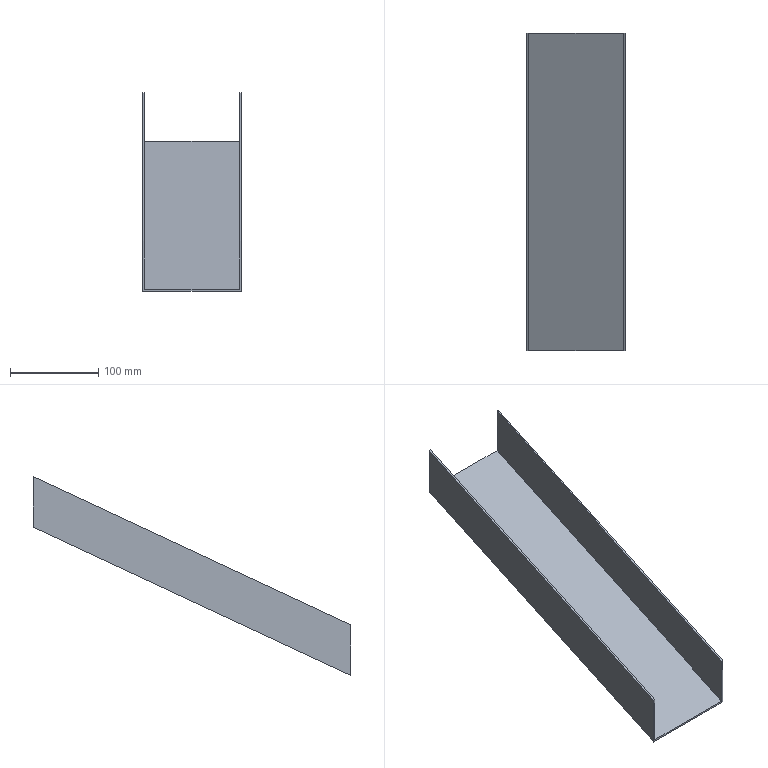Part | NX | features solid 2 | 1 solid | 10 faces | box 111.182 x 360 x 225.246 mm | volume 167770 mm3 | plane 10
STEP:
#1=CARTESIAN_POINT('',(100.,-105.,-113.856));
#2=VERTEX_POINT('',#1);
#3=CARTESIAN_POINT('',(102.,-105.,-113.856));
#4=VERTEX_POINT('',#3);
#5=CARTESIAN_POINT('',(121.182,-105.,-113.856));
#6=DIRECTION('',(-1.,0.,0.));
#7=VECTOR('',#6,1000.);
#8=LINE('',#5,#7);
#9=EDGE_CURVE('',#2,#4,#8,.F.);
#10=ORIENTED_EDGE('',*,*,#9,.F.);
#11=CARTESIAN_POINT('',(100.,-465.,-281.727));
#12=VERTEX_POINT('',#11);
#13=CARTESIAN_POINT('',(100.,-232.92,-173.506));
#14=DIRECTION('',(0.,-0.9063,-0.4226));
#15=VECTOR('',#14,1000.);
#16=LINE('',#13,#15);
#17=EDGE_CURVE('',#2,#12,#16,.T.);
#18=ORIENTED_EDGE('',*,*,#17,.T.);
#19=CARTESIAN_POINT('',(102.,-465.,-281.727));
#20=VERTEX_POINT('',#19);
#21=CARTESIAN_POINT('',(110.,-465.,-281.727));
#22=DIRECTION('',(-1.,0.,0.));
#23=VECTOR('',#22,1000.);
#24=LINE('',#21,#23);
#25=EDGE_CURVE('',#12,#20,#24,.F.);
#26=ORIENTED_EDGE('',*,*,#25,.T.);
#27=CARTESIAN_POINT('',(102.,-283.317,-197.007));
#28=DIRECTION('',(0.,-0.9063,-0.4226));
#29=VECTOR('',#28,1000.);
#30=LINE('',#27,#29);
#31=EDGE_CURVE('',#4,#20,#30,.T.);
#32=ORIENTED_EDGE('',*,*,#31,.F.);
#33=EDGE_LOOP('',(#10,#18,#26,#32));
#34=FACE_BOUND('',#33,.T.);
#35=CARTESIAN_POINT('',(110.,-161.131,-140.03));
#36=DIRECTION('',(0.,0.4226,-0.9063));
#37=DIRECTION('',(0.,-0.9063,-0.4226));
#38=AXIS2_PLACEMENT_3D('',#35,#36,#37);
#39=PLANE('',#38);
#40=ADVANCED_FACE('',(#34),#39,.F.);
#41=CARTESIAN_POINT('',(102.,-105.,-169.025));
#42=VERTEX_POINT('',#41);
#43=CARTESIAN_POINT('',(102.,-465.,-336.896));
#44=VERTEX_POINT('',#43);
#45=CARTESIAN_POINT('',(102.,-7.673,-123.64));
#46=DIRECTION('',(0.,-0.9063,-0.4226));
#47=VECTOR('',#46,1000.);
#48=LINE('',#45,#47);
#49=EDGE_CURVE('',#42,#44,#48,.T.);
#50=ORIENTED_EDGE('',*,*,#49,.F.);
#51=CARTESIAN_POINT('',(102.,-105.,0.000000171));
#52=DIRECTION('',(0.,0.,1.));
#53=VECTOR('',#52,1000.);
#54=LINE('',#51,#53);
#55=EDGE_CURVE('',#42,#4,#54,.T.);
#56=ORIENTED_EDGE('',*,*,#55,.T.);
#57=ORIENTED_EDGE('',*,*,#31,.T.);
#58=CARTESIAN_POINT('',(102.,-465.,-242.322));
#59=DIRECTION('',(0.,0.,1.));
#60=VECTOR('',#59,1000.);
#61=LINE('',#58,#60);
#62=EDGE_CURVE('',#44,#20,#61,.T.);
#63=ORIENTED_EDGE('',*,*,#62,.F.);
#64=EDGE_LOOP('',(#50,#56,#57,#63));
#65=FACE_BOUND('',#64,.T.);
#66=CARTESIAN_POINT('',(102.,-262.186,-242.322));
#67=DIRECTION('',(-1.,0.,0.));
#68=DIRECTION('',(0.,0.,1.));
#69=AXIS2_PLACEMENT_3D('',#66,#67,#68);
#70=PLANE('',#69);
#71=ADVANCED_FACE('',(#65),#70,.F.);
#72=ORIENTED_EDGE('',*,*,#55,.F.);
#73=CARTESIAN_POINT('',(209.182,-105.,-169.025));
#74=VERTEX_POINT('',#73);
#75=CARTESIAN_POINT('',(121.182,-105.,-169.025));
#76=DIRECTION('',(1.,0.,0.));
#77=VECTOR('',#76,1000.);
#78=LINE('',#75,#77);
#79=EDGE_CURVE('',#42,#74,#78,.T.);
#80=ORIENTED_EDGE('',*,*,#79,.T.);
#81=CARTESIAN_POINT('',(209.182,-105.,-113.856));
#82=VERTEX_POINT('',#81);
#83=CARTESIAN_POINT('',(209.182,-105.,0.000000171));
#84=DIRECTION('',(0.,0.,1.));
#85=VECTOR('',#84,1000.);
#86=LINE('',#83,#85);
#87=EDGE_CURVE('',#74,#82,#86,.T.);
#88=ORIENTED_EDGE('',*,*,#87,.T.);
#89=CARTESIAN_POINT('',(211.182,-105.,-113.856));
#90=VERTEX_POINT('',#89);
#91=CARTESIAN_POINT('',(211.182,-105.,-113.856));
#92=DIRECTION('',(1.,0.,0.));
#93=VECTOR('',#92,1000.);
#94=LINE('',#91,#93);
#95=EDGE_CURVE('',#82,#90,#94,.T.);
#96=ORIENTED_EDGE('',*,*,#95,.T.);
#97=CARTESIAN_POINT('',(211.182,-105.,-171.232));
#98=VERTEX_POINT('',#97);
#99=CARTESIAN_POINT('',(211.182,-105.,0.000000171));
#100=DIRECTION('',(0.,0.,1.));
#101=VECTOR('',#100,1000.);
#102=LINE('',#99,#101);
#103=EDGE_CURVE('',#98,#90,#102,.T.);
#104=ORIENTED_EDGE('',*,*,#103,.F.);
#105=CARTESIAN_POINT('',(100.,-105.,-171.232));
#106=VERTEX_POINT('',#105);
#107=CARTESIAN_POINT('',(540.,-105.,-171.232));
#108=DIRECTION('',(1.,0.,0.));
#109=VECTOR('',#108,1000.);
#110=LINE('',#107,#109);
#111=EDGE_CURVE('',#106,#98,#110,.T.);
#112=ORIENTED_EDGE('',*,*,#111,.F.);
#113=CARTESIAN_POINT('',(100.,-105.,0.000000171));
#114=DIRECTION('',(0.,0.,1.));
#115=VECTOR('',#114,1000.);
#116=LINE('',#113,#115);
#117=EDGE_CURVE('',#106,#2,#116,.T.);
#118=ORIENTED_EDGE('',*,*,#117,.T.);
#119=ORIENTED_EDGE('',*,*,#9,.T.);
#120=EDGE_LOOP('',(#72,#80,#88,#96,#104,#112,#118,#119));
#121=FACE_BOUND('',#120,.T.);
#122=CARTESIAN_POINT('',(121.182,-105.,0.000000171));
#123=DIRECTION('',(0.,1.,0.));
#124=DIRECTION('',(0.,0.,1.));
#125=AXIS2_PLACEMENT_3D('',#122,#123,#124);
#126=PLANE('',#125);
#127=ADVANCED_FACE('',(#121),#126,.T.);
#128=ORIENTED_EDGE('',*,*,#17,.F.);
#129=ORIENTED_EDGE('',*,*,#117,.F.);
#130=CARTESIAN_POINT('',(100.,-465.,-339.102));
#131=VERTEX_POINT('',#130);
#132=CARTESIAN_POINT('',(100.,-6.828,-125.453));
#133=DIRECTION('',(0.,0.9063,0.4226));
#134=VECTOR('',#133,1000.);
#135=LINE('',#132,#134);
#136=EDGE_CURVE('',#131,#106,#135,.T.);
#137=ORIENTED_EDGE('',*,*,#136,.F.);
#138=CARTESIAN_POINT('',(100.,-465.,-85.));
#139=DIRECTION('',(0.,0.,-1.));
#140=VECTOR('',#139,1000.);
#141=LINE('',#138,#140);
#142=EDGE_CURVE('',#12,#131,#141,.T.);
#143=ORIENTED_EDGE('',*,*,#142,.F.);
#144=EDGE_LOOP('',(#128,#129,#137,#143));
#145=FACE_BOUND('',#144,.T.);
#146=CARTESIAN_POINT('',(100.,-90.,-480.));
#147=DIRECTION('',(-1.,0.,0.));
#148=DIRECTION('',(0.,0.,1.));
#149=AXIS2_PLACEMENT_3D('',#146,#147,#148);
#150=PLANE('',#149);
#151=ADVANCED_FACE('',(#145),#150,.T.);
#152=CARTESIAN_POINT('',(211.182,-465.,-339.102));
#153=VERTEX_POINT('',#152);
#154=CARTESIAN_POINT('',(-910.,-465.,-339.102));
#155=DIRECTION('',(1.,0.,0.));
#156=VECTOR('',#155,1000.);
#157=LINE('',#154,#156);
#158=EDGE_CURVE('',#131,#153,#157,.T.);
#159=ORIENTED_EDGE('',*,*,#158,.T.);
#160=CARTESIAN_POINT('',(211.182,-465.,-281.727));
#161=VERTEX_POINT('',#160);
#162=CARTESIAN_POINT('',(211.182,-465.,-85.));
#163=DIRECTION('',(0.,0.,-1.));
#164=VECTOR('',#163,1000.);
#165=LINE('',#162,#164);
#166=EDGE_CURVE('',#161,#153,#165,.T.);
#167=ORIENTED_EDGE('',*,*,#166,.F.);
#168=CARTESIAN_POINT('',(209.182,-465.,-281.727));
#169=VERTEX_POINT('',#168);
#170=CARTESIAN_POINT('',(211.182,-465.,-281.727));
#171=DIRECTION('',(-1.,0.,0.));
#172=VECTOR('',#171,1000.);
#173=LINE('',#170,#172);
#174=EDGE_CURVE('',#161,#169,#173,.T.);
#175=ORIENTED_EDGE('',*,*,#174,.T.);
#176=CARTESIAN_POINT('',(209.182,-465.,-336.896));
#177=VERTEX_POINT('',#176);
#178=CARTESIAN_POINT('',(209.182,-465.,-85.));
#179=DIRECTION('',(0.,0.,-1.));
#180=VECTOR('',#179,1000.);
#181=LINE('',#178,#180);
#182=EDGE_CURVE('',#169,#177,#181,.T.);
#183=ORIENTED_EDGE('',*,*,#182,.T.);
#184=CARTESIAN_POINT('',(140.,-465.,-336.896));
#185=DIRECTION('',(1.,0.,0.));
#186=VECTOR('',#185,1000.);
#187=LINE('',#184,#186);
#188=EDGE_CURVE('',#44,#177,#187,.T.);
#189=ORIENTED_EDGE('',*,*,#188,.F.);
#190=ORIENTED_EDGE('',*,*,#62,.T.);
#191=ORIENTED_EDGE('',*,*,#25,.F.);
#192=ORIENTED_EDGE('',*,*,#142,.T.);
#193=EDGE_LOOP('',(#159,#167,#175,#183,#189,#190,#191,#192));
#194=FACE_BOUND('',#193,.T.);
#195=CARTESIAN_POINT('',(-910.,-465.,-85.));
#196=DIRECTION('',(0.,-1.,0.));
#197=DIRECTION('',(0.,0.,-1.));
#198=AXIS2_PLACEMENT_3D('',#195,#196,#197);
#199=PLANE('',#198);
#200=ADVANCED_FACE('',(#194),#199,.T.);
#201=ORIENTED_EDGE('',*,*,#136,.T.);
#202=ORIENTED_EDGE('',*,*,#111,.T.);
#203=CARTESIAN_POINT('',(211.182,-6.828,-125.453));
#204=DIRECTION('',(0.,0.9063,0.4226));
#205=VECTOR('',#204,1000.);
#206=LINE('',#203,#205);
#207=EDGE_CURVE('',#153,#98,#206,.T.);
#208=ORIENTED_EDGE('',*,*,#207,.F.);
#209=ORIENTED_EDGE('',*,*,#158,.F.);
#210=EDGE_LOOP('',(#201,#202,#208,#209));
#211=FACE_BOUND('',#210,.T.);
#212=CARTESIAN_POINT('',(540.,-6.828,-125.453));
#213=DIRECTION('',(0.,0.4226,-0.9063));
#214=DIRECTION('',(0.,0.9063,0.4226));
#215=AXIS2_PLACEMENT_3D('',#212,#213,#214);
#216=PLANE('',#215);
#217=ADVANCED_FACE('',(#211),#216,.T.);
#218=ORIENTED_EDGE('',*,*,#188,.T.);
#219=CARTESIAN_POINT('',(209.182,-7.673,-123.64));
#220=DIRECTION('',(0.,-0.9063,-0.4226));
#221=VECTOR('',#220,1000.);
#222=LINE('',#219,#221);
#223=EDGE_CURVE('',#74,#177,#222,.T.);
#224=ORIENTED_EDGE('',*,*,#223,.F.);
#225=ORIENTED_EDGE('',*,*,#79,.F.);
#226=ORIENTED_EDGE('',*,*,#49,.T.);
#227=EDGE_LOOP('',(#218,#224,#225,#226));
#228=FACE_BOUND('',#227,.T.);
#229=CARTESIAN_POINT('',(140.,-7.673,-123.64));
#230=DIRECTION('',(0.,-0.4226,0.9063));
#231=DIRECTION('',(0.,-0.9063,-0.4226));
#232=AXIS2_PLACEMENT_3D('',#229,#230,#231);
#233=PLANE('',#232);
#234=ADVANCED_FACE('',(#228),#233,.T.);
#235=CARTESIAN_POINT('',(211.182,-57.284,-91.605));
#236=DIRECTION('',(0.,-0.9063,-0.4226));
#237=VECTOR('',#236,1000.);
#238=LINE('',#235,#237);
#239=EDGE_CURVE('',#90,#161,#238,.T.);
#240=ORIENTED_EDGE('',*,*,#239,.T.);
#241=ORIENTED_EDGE('',*,*,#166,.T.);
#242=ORIENTED_EDGE('',*,*,#207,.T.);
#243=ORIENTED_EDGE('',*,*,#103,.T.);
#244=EDGE_LOOP('',(#240,#241,#242,#243));
#245=FACE_BOUND('',#244,.T.);
#246=CARTESIAN_POINT('',(211.182,-100.,0.000000167));
#247=DIRECTION('',(-1.,0.,0.));
#248=DIRECTION('',(0.,-1.,0.));
#249=AXIS2_PLACEMENT_3D('',#246,#247,#248);
#250=PLANE('',#249);
#251=ADVANCED_FACE('',(#245),#250,.F.);
#252=CARTESIAN_POINT('',(209.182,-57.284,-91.605));
#253=DIRECTION('',(0.,-0.9063,-0.4226));
#254=VECTOR('',#253,1000.);
#255=LINE('',#252,#254);
#256=EDGE_CURVE('',#82,#169,#255,.T.);
#257=ORIENTED_EDGE('',*,*,#256,.T.);
#258=ORIENTED_EDGE('',*,*,#174,.F.);
#259=ORIENTED_EDGE('',*,*,#239,.F.);
#260=ORIENTED_EDGE('',*,*,#95,.F.);
#261=EDGE_LOOP('',(#257,#258,#259,#260));
#262=FACE_BOUND('',#261,.T.);
#263=CARTESIAN_POINT('',(211.182,-28.804,-78.325));
#264=DIRECTION('',(0.,0.4226,-0.9063));
#265=DIRECTION('',(0.,0.9063,0.4226));
#266=AXIS2_PLACEMENT_3D('',#263,#264,#265);
#267=PLANE('',#266);
#268=ADVANCED_FACE('',(#262),#267,.F.);
#269=ORIENTED_EDGE('',*,*,#223,.T.);
#270=ORIENTED_EDGE('',*,*,#182,.F.);
#271=ORIENTED_EDGE('',*,*,#256,.F.);
#272=ORIENTED_EDGE('',*,*,#87,.F.);
#273=EDGE_LOOP('',(#269,#270,#271,#272));
#274=FACE_BOUND('',#273,.T.);
#275=CARTESIAN_POINT('',(209.182,-100.,0.000000167));
#276=DIRECTION('',(-1.,0.,0.));
#277=DIRECTION('',(0.,-1.,0.));
#278=AXIS2_PLACEMENT_3D('',#275,#276,#277);
#279=PLANE('',#278);
#280=ADVANCED_FACE('',(#274),#279,.T.);
#281=CLOSED_SHELL('',(#40,#71,#127,#151,#200,#217,#234,#251,#268,#280));
#282=MANIFOLD_SOLID_BREP('',#281);
#283=(LENGTH_UNIT()NAMED_UNIT(*)SI_UNIT(.MILLI.,.METRE.));
#284=UNCERTAINTY_MEASURE_WITH_UNIT(LENGTH_MEASURE(0.00001),#283,'','');
#285=(NAMED_UNIT(*)PLANE_ANGLE_UNIT()SI_UNIT($,.RADIAN.));
#286=(NAMED_UNIT(*)SI_UNIT($,.STERADIAN.)SOLID_ANGLE_UNIT());
#287=(GEOMETRIC_REPRESENTATION_CONTEXT(3)GLOBAL_UNCERTAINTY_ASSIGNED_CONTEXT((#284))GLOBAL_UNIT_ASSIGNED_CONTEXT((#283,#285,#286))REPRESENTATION_CONTEXT('',''));
#288=ADVANCED_BREP_SHAPE_REPRESENTATION('',(#282),#287);